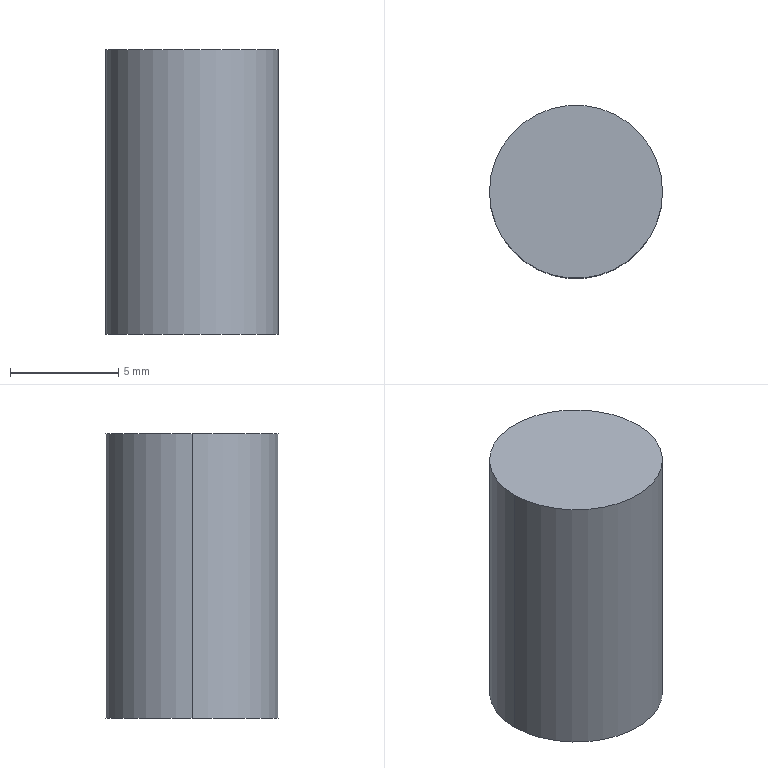Part | SolidWorks | features BaseBody 1 | 1 solid | 4 faces | box 8 x 8 x 13.146 mm | volume 660.8 mm3 | cylinder 2 | plane 2 | commonest cylinder face diameters 8 x2
STEP:
#1=CARTESIAN_POINT('',(-4.,0.,372.146));
#2=VERTEX_POINT('',#1);
#3=CARTESIAN_POINT('',(4.,0.,372.146));
#4=VERTEX_POINT('',#3);
#5=CARTESIAN_POINT('',(0.,0.,372.146));
#6=DIRECTION('',(0.,0.,-1.));
#7=DIRECTION('',(-1.,0.,0.));
#8=AXIS2_PLACEMENT_3D('',#5,#6,#7);
#9=CIRCLE('',#8,4.);
#10=EDGE_CURVE('',#2,#4,#9,.T.);
#11=ORIENTED_EDGE('',*,*,#10,.T.);
#12=CARTESIAN_POINT('',(4.,0.,359.));
#13=VERTEX_POINT('',#12);
#14=CARTESIAN_POINT('',(4.,0.,372.146));
#15=DIRECTION('',(0.,0.,-1.));
#16=VECTOR('',#15,1000.);
#17=LINE('',#14,#16);
#18=EDGE_CURVE('',#4,#13,#17,.T.);
#19=ORIENTED_EDGE('',*,*,#18,.T.);
#20=CARTESIAN_POINT('',(-4.,0.,359.));
#21=VERTEX_POINT('',#20);
#22=CARTESIAN_POINT('',(0.,0.,359.));
#23=DIRECTION('',(0.,0.,1.));
#24=DIRECTION('',(-1.,0.,0.));
#25=AXIS2_PLACEMENT_3D('',#22,#23,#24);
#26=CIRCLE('',#25,4.);
#27=EDGE_CURVE('',#13,#21,#26,.T.);
#28=ORIENTED_EDGE('',*,*,#27,.T.);
#29=CARTESIAN_POINT('',(-4.,0.,372.146));
#30=DIRECTION('',(0.,0.,-1.));
#31=VECTOR('',#30,1000.);
#32=LINE('',#29,#31);
#33=EDGE_CURVE('',#2,#21,#32,.T.);
#34=ORIENTED_EDGE('',*,*,#33,.F.);
#35=EDGE_LOOP('',(#11,#19,#28,#34));
#36=FACE_OUTER_BOUND('',#35,.T.);
#37=CARTESIAN_POINT('',(0.,0.,372.146));
#38=DIRECTION('',(0.,0.,-1.));
#39=DIRECTION('',(-1.,0.,0.));
#40=AXIS2_PLACEMENT_3D('',#37,#38,#39);
#41=CYLINDRICAL_SURFACE('',#40,4.);
#42=ADVANCED_FACE('',(#36),#41,.T.);
#43=ORIENTED_EDGE('',*,*,#18,.F.);
#44=CARTESIAN_POINT('',(0.,0.,372.146));
#45=DIRECTION('',(0.,0.,-1.));
#46=DIRECTION('',(-1.,0.,0.));
#47=AXIS2_PLACEMENT_3D('',#44,#45,#46);
#48=CIRCLE('',#47,4.);
#49=EDGE_CURVE('',#4,#2,#48,.T.);
#50=ORIENTED_EDGE('',*,*,#49,.T.);
#51=ORIENTED_EDGE('',*,*,#33,.T.);
#52=CARTESIAN_POINT('',(0.,0.,359.));
#53=DIRECTION('',(0.,0.,1.));
#54=DIRECTION('',(-1.,0.,0.));
#55=AXIS2_PLACEMENT_3D('',#52,#53,#54);
#56=CIRCLE('',#55,4.);
#57=EDGE_CURVE('',#21,#13,#56,.T.);
#58=ORIENTED_EDGE('',*,*,#57,.T.);
#59=EDGE_LOOP('',(#43,#50,#51,#58));
#60=FACE_OUTER_BOUND('',#59,.T.);
#61=CARTESIAN_POINT('',(0.,0.,372.146));
#62=DIRECTION('',(0.,0.,-1.));
#63=DIRECTION('',(-1.,0.,0.));
#64=AXIS2_PLACEMENT_3D('',#61,#62,#63);
#65=CYLINDRICAL_SURFACE('',#64,4.);
#66=ADVANCED_FACE('',(#60),#65,.T.);
#67=ORIENTED_EDGE('',*,*,#10,.F.);
#68=ORIENTED_EDGE('',*,*,#49,.F.);
#69=EDGE_LOOP('',(#67,#68));
#70=FACE_OUTER_BOUND('',#69,.T.);
#71=CARTESIAN_POINT('',(0.,0.,372.146));
#72=DIRECTION('',(0.,0.,1.));
#73=DIRECTION('',(1.,0.,0.));
#74=AXIS2_PLACEMENT_3D('',#71,#72,#73);
#75=PLANE('',#74);
#76=ADVANCED_FACE('',(#70),#75,.T.);
#77=ORIENTED_EDGE('',*,*,#57,.F.);
#78=ORIENTED_EDGE('',*,*,#27,.F.);
#79=EDGE_LOOP('',(#77,#78));
#80=FACE_OUTER_BOUND('',#79,.T.);
#81=CARTESIAN_POINT('',(0.,0.,359.));
#82=DIRECTION('',(0.,0.,1.));
#83=DIRECTION('',(1.,0.,0.));
#84=AXIS2_PLACEMENT_3D('',#81,#82,#83);
#85=PLANE('',#84);
#86=ADVANCED_FACE('',(#80),#85,.F.);
#87=CLOSED_SHELL('',(#42,#66,#76,#86));
#88=MANIFOLD_SOLID_BREP('',#87);
#89=CARTESIAN_POINT('',(0.,0.,0.));
#90=DIRECTION('',(0.,0.,1.));
#91=DIRECTION('',(1.,0.,0.));
#92=AXIS2_PLACEMENT_3D('',#89,#90,#91);
#93=(LENGTH_UNIT()NAMED_UNIT(*)SI_UNIT(.MILLI.,.METRE.));
#94=UNCERTAINTY_MEASURE_WITH_UNIT(LENGTH_MEASURE(0.00001),#93,'','');
#95=(NAMED_UNIT(*)PLANE_ANGLE_UNIT()SI_UNIT($,.RADIAN.));
#96=(NAMED_UNIT(*)SI_UNIT($,.STERADIAN.)SOLID_ANGLE_UNIT());
#97=(GEOMETRIC_REPRESENTATION_CONTEXT(3)GLOBAL_UNCERTAINTY_ASSIGNED_CONTEXT((#94))GLOBAL_UNIT_ASSIGNED_CONTEXT((#93,#95,#96))REPRESENTATION_CONTEXT('',''));
#98=ADVANCED_BREP_SHAPE_REPRESENTATION('',(#88,#92),#97);